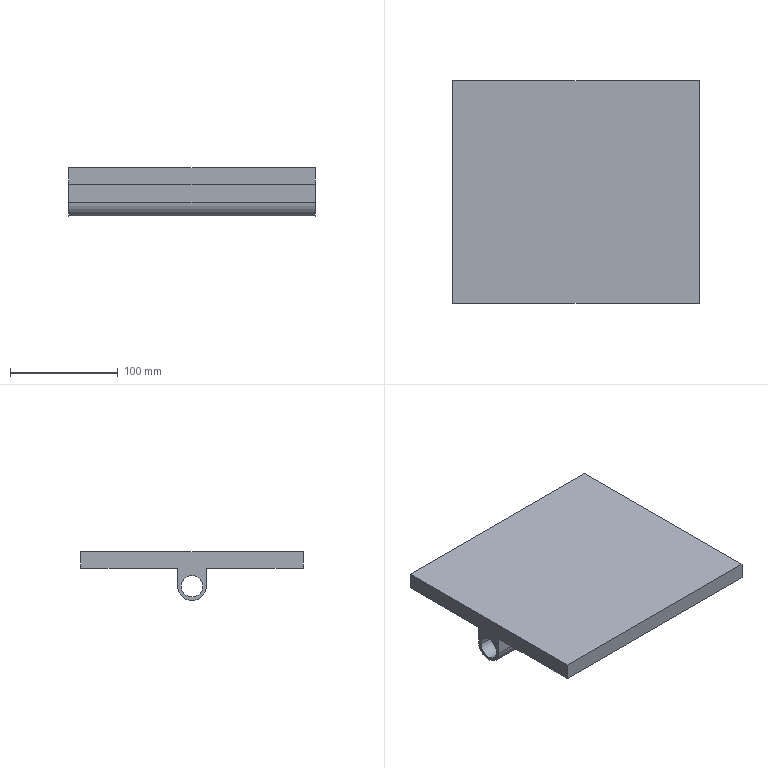Part | STEP file | 1 solid | 12 faces | box 229 x 206.363 x 45.369 mm | volume 819761 mm3 | plane 9 | cylinder 3 | commonest cylinder face diameters 20 x2 26.524 x1
STEP:
#1=CARTESIAN_POINT('',(0.,0.,0.));
#2=DIRECTION('',(0.,0.,1.));
#3=DIRECTION('',(1.,0.,0.));
#4=AXIS2_PLACEMENT_3D('',#1,#2,#3);
#5=CARTESIAN_POINT('',(226.149,563.5,104.906));
#6=VERTEX_POINT('',#5);
#7=CARTESIAN_POINT('',(455.149,563.5,104.906));
#8=VERTEX_POINT('',#7);
#9=CARTESIAN_POINT('',(226.149,563.5,104.906));
#10=DIRECTION('',(1.,0.,0.));
#11=VECTOR('',#10,1.);
#12=LINE('',#9,#11);
#13=CARTESIAN_POINT('',(226.149,553.5,104.906));
#14=DIRECTION('',(1.,0.,0.));
#15=DIRECTION('',(0.,1.,0.));
#16=AXIS2_PLACEMENT_3D('',#13,#14,#15);
#17=CYLINDRICAL_SURFACE('',#16,10.);
#18=CARTESIAN_POINT('',(6.283,0.));
#19=DIRECTION('',(0.,1.));
#20=VECTOR('',#19,1.);
#21=LINE('',#18,#20);
#22=(GEOMETRIC_REPRESENTATION_CONTEXT(2)PARAMETRIC_REPRESENTATION_CONTEXT()REPRESENTATION_CONTEXT('',''));
#23=DEFINITIONAL_REPRESENTATION('',(#21),#22);
#24=PCURVE('',#17,#23);
#25=CARTESIAN_POINT('',(226.149,553.5,104.906));
#26=DIRECTION('',(1.,0.,0.));
#27=DIRECTION('',(0.,1.,0.));
#28=AXIS2_PLACEMENT_3D('',#25,#26,#27);
#29=CYLINDRICAL_SURFACE('',#28,10.);
#30=CARTESIAN_POINT('',(0.,0.));
#31=DIRECTION('',(0.,1.));
#32=VECTOR('',#31,1.);
#33=LINE('',#30,#32);
#34=(GEOMETRIC_REPRESENTATION_CONTEXT(2)PARAMETRIC_REPRESENTATION_CONTEXT()REPRESENTATION_CONTEXT('',''));
#35=DEFINITIONAL_REPRESENTATION('',(#33),#34);
#36=PCURVE('',#29,#35);
#37=SURFACE_CURVE('',#12,(#24,#36),.PCURVE_S1.);
#38=EDGE_CURVE('',#6,#8,#37,.T.);
#39=ORIENTED_EDGE('',*,*,#38,.T.);
#40=CARTESIAN_POINT('',(455.149,543.5,104.906));
#41=VERTEX_POINT('',#40);
#42=CARTESIAN_POINT('',(455.149,553.5,104.906));
#43=DIRECTION('',(-1.,0.,0.));
#44=DIRECTION('',(0.,-1.,0.));
#45=AXIS2_PLACEMENT_3D('',#42,#43,#44);
#46=CIRCLE('',#45,10.);
#47=CARTESIAN_POINT('',(9.425,229.));
#48=DIRECTION('',(-1.,0.));
#49=VECTOR('',#48,1.);
#50=LINE('',#47,#49);
#51=(GEOMETRIC_REPRESENTATION_CONTEXT(2)PARAMETRIC_REPRESENTATION_CONTEXT()REPRESENTATION_CONTEXT('',''));
#52=DEFINITIONAL_REPRESENTATION('',(#50),#51);
#53=PCURVE('',#17,#52);
#54=CARTESIAN_POINT('',(455.149,553.5,104.906));
#55=DIRECTION('',(-1.,0.,0.));
#56=DIRECTION('',(0.,-1.,0.));
#57=AXIS2_PLACEMENT_3D('',#54,#55,#56);
#58=PLANE('',#57);
#59=CARTESIAN_POINT('',(0.,0.));
#60=DIRECTION('',(1.,0.));
#61=AXIS2_PLACEMENT_2D('',#59,#60);
#62=CIRCLE('',#61,10.);
#63=(GEOMETRIC_REPRESENTATION_CONTEXT(2)PARAMETRIC_REPRESENTATION_CONTEXT()REPRESENTATION_CONTEXT('',''));
#64=DEFINITIONAL_REPRESENTATION('',(#62),#63);
#65=PCURVE('',#58,#64);
#66=SURFACE_CURVE('',#46,(#53,#65),.PCURVE_S1.);
#67=EDGE_CURVE('',#8,#41,#66,.T.);
#68=ORIENTED_EDGE('',*,*,#67,.T.);
#69=CARTESIAN_POINT('',(226.149,543.5,104.906));
#70=VERTEX_POINT('',#69);
#71=CARTESIAN_POINT('',(226.149,543.5,104.906));
#72=DIRECTION('',(1.,0.,0.));
#73=VECTOR('',#72,1.);
#74=LINE('',#71,#73);
#75=CARTESIAN_POINT('',(3.142,0.));
#76=DIRECTION('',(0.,1.));
#77=VECTOR('',#76,1.);
#78=LINE('',#75,#77);
#79=(GEOMETRIC_REPRESENTATION_CONTEXT(2)PARAMETRIC_REPRESENTATION_CONTEXT()REPRESENTATION_CONTEXT('',''));
#80=DEFINITIONAL_REPRESENTATION('',(#78),#79);
#81=PCURVE('',#17,#80);
#82=CARTESIAN_POINT('',(3.142,0.));
#83=DIRECTION('',(0.,1.));
#84=VECTOR('',#83,1.);
#85=LINE('',#82,#84);
#86=(GEOMETRIC_REPRESENTATION_CONTEXT(2)PARAMETRIC_REPRESENTATION_CONTEXT()REPRESENTATION_CONTEXT('',''));
#87=DEFINITIONAL_REPRESENTATION('',(#85),#86);
#88=PCURVE('',#29,#87);
#89=SURFACE_CURVE('',#74,(#81,#88),.PCURVE_S1.);
#90=EDGE_CURVE('',#70,#41,#89,.T.);
#91=ORIENTED_EDGE('',*,*,#90,.F.);
#92=CARTESIAN_POINT('',(226.149,553.5,104.906));
#93=DIRECTION('',(-1.,0.,0.));
#94=DIRECTION('',(0.,-1.,0.));
#95=AXIS2_PLACEMENT_3D('',#92,#93,#94);
#96=CIRCLE('',#95,10.);
#97=CARTESIAN_POINT('',(9.425,0.));
#98=DIRECTION('',(-1.,0.));
#99=VECTOR('',#98,1.);
#100=LINE('',#97,#99);
#101=(GEOMETRIC_REPRESENTATION_CONTEXT(2)PARAMETRIC_REPRESENTATION_CONTEXT()REPRESENTATION_CONTEXT('',''));
#102=DEFINITIONAL_REPRESENTATION('',(#100),#101);
#103=PCURVE('',#17,#102);
#104=CARTESIAN_POINT('',(226.149,553.5,104.906));
#105=DIRECTION('',(-1.,0.,0.));
#106=DIRECTION('',(0.,-1.,0.));
#107=AXIS2_PLACEMENT_3D('',#104,#105,#106);
#108=PLANE('',#107);
#109=CARTESIAN_POINT('',(0.,0.));
#110=DIRECTION('',(1.,0.));
#111=AXIS2_PLACEMENT_2D('',#109,#110);
#112=CIRCLE('',#111,10.);
#113=(GEOMETRIC_REPRESENTATION_CONTEXT(2)PARAMETRIC_REPRESENTATION_CONTEXT()REPRESENTATION_CONTEXT('',''));
#114=DEFINITIONAL_REPRESENTATION('',(#112),#113);
#115=PCURVE('',#108,#114);
#116=SURFACE_CURVE('',#96,(#103,#115),.PCURVE_S1.);
#117=EDGE_CURVE('',#6,#70,#116,.T.);
#118=ORIENTED_EDGE('',*,*,#117,.F.);
#119=EDGE_LOOP('',(#39,#68,#91,#118));
#120=FACE_BOUND('',#119,.F.);
#121=ADVANCED_FACE('',(#120),#17,.F.);
#122=CARTESIAN_POINT('',(226.149,656.681,121.632));
#123=VERTEX_POINT('',#122);
#124=CARTESIAN_POINT('',(226.149,566.762,121.632));
#125=VERTEX_POINT('',#124);
#126=CARTESIAN_POINT('',(226.149,656.681,121.632));
#127=DIRECTION('',(0.,-1.,0.));
#128=VECTOR('',#127,1.);
#129=LINE('',#126,#128);
#130=CARTESIAN_POINT('',(-103.181,16.727));
#131=DIRECTION('',(1.,0.));
#132=VECTOR('',#131,1.);
#133=LINE('',#130,#132);
#134=(GEOMETRIC_REPRESENTATION_CONTEXT(2)PARAMETRIC_REPRESENTATION_CONTEXT()REPRESENTATION_CONTEXT('',''));
#135=DEFINITIONAL_REPRESENTATION('',(#133),#134);
#136=PCURVE('',#108,#135);
#137=CARTESIAN_POINT('',(226.149,656.681,121.632));
#138=DIRECTION('',(0.,0.,1.));
#139=DIRECTION('',(0.,-1.,0.));
#140=AXIS2_PLACEMENT_3D('',#137,#138,#139);
#141=PLANE('',#140);
#142=CARTESIAN_POINT('',(0.,0.));
#143=DIRECTION('',(1.,0.));
#144=VECTOR('',#143,1.);
#145=LINE('',#142,#144);
#146=(GEOMETRIC_REPRESENTATION_CONTEXT(2)PARAMETRIC_REPRESENTATION_CONTEXT()REPRESENTATION_CONTEXT('',''));
#147=DEFINITIONAL_REPRESENTATION('',(#145),#146);
#148=PCURVE('',#141,#147);
#149=SURFACE_CURVE('',#129,(#136,#148),.PCURVE_S1.);
#150=EDGE_CURVE('',#123,#125,#149,.T.);
#151=ORIENTED_EDGE('',*,*,#150,.T.);
#152=CARTESIAN_POINT('',(226.149,566.762,104.906));
#153=VERTEX_POINT('',#152);
#154=CARTESIAN_POINT('',(226.149,566.762,104.906));
#155=DIRECTION('',(0.,0.,-1.));
#156=VECTOR('',#155,1.);
#157=LINE('',#154,#156);
#158=CARTESIAN_POINT('',(-13.262,0.));
#159=DIRECTION('',(0.,-1.));
#160=VECTOR('',#159,1.);
#161=LINE('',#158,#160);
#162=(GEOMETRIC_REPRESENTATION_CONTEXT(2)PARAMETRIC_REPRESENTATION_CONTEXT()REPRESENTATION_CONTEXT('',''));
#163=DEFINITIONAL_REPRESENTATION('',(#161),#162);
#164=PCURVE('',#108,#163);
#165=CARTESIAN_POINT('',(226.149,566.762,104.906));
#166=DIRECTION('',(0.,-1.,0.));
#167=DIRECTION('',(1.,0.,0.));
#168=AXIS2_PLACEMENT_3D('',#165,#166,#167);
#169=PLANE('',#168);
#170=CARTESIAN_POINT('',(0.,0.));
#171=DIRECTION('',(0.,-1.));
#172=VECTOR('',#171,1.);
#173=LINE('',#170,#172);
#174=(GEOMETRIC_REPRESENTATION_CONTEXT(2)PARAMETRIC_REPRESENTATION_CONTEXT()REPRESENTATION_CONTEXT('',''));
#175=DEFINITIONAL_REPRESENTATION('',(#173),#174);
#176=PCURVE('',#169,#175);
#177=SURFACE_CURVE('',#157,(#164,#176),.PCURVE_S1.);
#178=EDGE_CURVE('',#125,#153,#177,.T.);
#179=ORIENTED_EDGE('',*,*,#178,.T.);
#180=CARTESIAN_POINT('',(226.149,540.238,104.906));
#181=VERTEX_POINT('',#180);
#182=CARTESIAN_POINT('',(226.149,553.5,104.906));
#183=DIRECTION('',(-1.,0.,0.));
#184=DIRECTION('',(0.,-1.,0.));
#185=AXIS2_PLACEMENT_3D('',#182,#183,#184);
#186=CIRCLE('',#185,13.262);
#187=CARTESIAN_POINT('',(0.,0.));
#188=DIRECTION('',(1.,0.));
#189=AXIS2_PLACEMENT_2D('',#187,#188);
#190=CIRCLE('',#189,13.262);
#191=(GEOMETRIC_REPRESENTATION_CONTEXT(2)PARAMETRIC_REPRESENTATION_CONTEXT()REPRESENTATION_CONTEXT('',''));
#192=DEFINITIONAL_REPRESENTATION('',(#190),#191);
#193=PCURVE('',#108,#192);
#194=CARTESIAN_POINT('',(226.149,553.5,104.906));
#195=DIRECTION('',(1.,0.,0.));
#196=DIRECTION('',(0.,1.,0.));
#197=AXIS2_PLACEMENT_3D('',#194,#195,#196);
#198=CYLINDRICAL_SURFACE('',#197,13.262);
#199=CARTESIAN_POINT('',(9.425,0.));
#200=DIRECTION('',(-1.,0.));
#201=VECTOR('',#200,1.);
#202=LINE('',#199,#201);
#203=(GEOMETRIC_REPRESENTATION_CONTEXT(2)PARAMETRIC_REPRESENTATION_CONTEXT()REPRESENTATION_CONTEXT('',''));
#204=DEFINITIONAL_REPRESENTATION('',(#202),#203);
#205=PCURVE('',#198,#204);
#206=SURFACE_CURVE('',#186,(#193,#205),.PCURVE_S1.);
#207=EDGE_CURVE('',#153,#181,#206,.T.);
#208=ORIENTED_EDGE('',*,*,#207,.T.);
#209=CARTESIAN_POINT('',(226.149,540.238,121.632));
#210=VERTEX_POINT('',#209);
#211=CARTESIAN_POINT('',(226.149,540.238,104.906));
#212=DIRECTION('',(0.,0.,1.));
#213=VECTOR('',#212,1.);
#214=LINE('',#211,#213);
#215=CARTESIAN_POINT('',(13.262,0.));
#216=DIRECTION('',(0.,1.));
#217=VECTOR('',#216,1.);
#218=LINE('',#215,#217);
#219=(GEOMETRIC_REPRESENTATION_CONTEXT(2)PARAMETRIC_REPRESENTATION_CONTEXT()REPRESENTATION_CONTEXT('',''));
#220=DEFINITIONAL_REPRESENTATION('',(#218),#219);
#221=PCURVE('',#108,#220);
#222=CARTESIAN_POINT('',(226.149,540.238,104.906));
#223=DIRECTION('',(0.,1.,0.));
#224=DIRECTION('',(-1.,0.,0.));
#225=AXIS2_PLACEMENT_3D('',#222,#223,#224);
#226=PLANE('',#225);
#227=CARTESIAN_POINT('',(0.,0.));
#228=DIRECTION('',(0.,1.));
#229=VECTOR('',#228,1.);
#230=LINE('',#227,#229);
#231=(GEOMETRIC_REPRESENTATION_CONTEXT(2)PARAMETRIC_REPRESENTATION_CONTEXT()REPRESENTATION_CONTEXT('',''));
#232=DEFINITIONAL_REPRESENTATION('',(#230),#231);
#233=PCURVE('',#226,#232);
#234=SURFACE_CURVE('',#214,(#221,#233),.PCURVE_S1.);
#235=EDGE_CURVE('',#181,#210,#234,.T.);
#236=ORIENTED_EDGE('',*,*,#235,.T.);
#237=CARTESIAN_POINT('',(226.149,450.319,121.632));
#238=VERTEX_POINT('',#237);
#239=CARTESIAN_POINT('',(226.149,540.238,121.632));
#240=DIRECTION('',(0.,-1.,0.));
#241=VECTOR('',#240,1.);
#242=LINE('',#239,#241);
#243=CARTESIAN_POINT('',(13.262,16.727));
#244=DIRECTION('',(1.,0.));
#245=VECTOR('',#244,1.);
#246=LINE('',#243,#245);
#247=(GEOMETRIC_REPRESENTATION_CONTEXT(2)PARAMETRIC_REPRESENTATION_CONTEXT()REPRESENTATION_CONTEXT('',''));
#248=DEFINITIONAL_REPRESENTATION('',(#246),#247);
#249=PCURVE('',#108,#248);
#250=CARTESIAN_POINT('',(226.149,540.238,121.632));
#251=DIRECTION('',(0.,0.,1.));
#252=DIRECTION('',(0.,-1.,0.));
#253=AXIS2_PLACEMENT_3D('',#250,#251,#252);
#254=PLANE('',#253);
#255=CARTESIAN_POINT('',(0.,0.));
#256=DIRECTION('',(1.,0.));
#257=VECTOR('',#256,1.);
#258=LINE('',#255,#257);
#259=(GEOMETRIC_REPRESENTATION_CONTEXT(2)PARAMETRIC_REPRESENTATION_CONTEXT()REPRESENTATION_CONTEXT('',''));
#260=DEFINITIONAL_REPRESENTATION('',(#258),#259);
#261=PCURVE('',#254,#260);
#262=SURFACE_CURVE('',#242,(#249,#261),.PCURVE_S1.);
#263=EDGE_CURVE('',#210,#238,#262,.T.);
#264=ORIENTED_EDGE('',*,*,#263,.T.);
#265=CARTESIAN_POINT('',(226.149,450.319,137.013));
#266=VERTEX_POINT('',#265);
#267=CARTESIAN_POINT('',(226.149,450.319,121.632));
#268=DIRECTION('',(0.,0.,1.));
#269=VECTOR('',#268,1.);
#270=LINE('',#267,#269);
#271=CARTESIAN_POINT('',(103.181,16.727));
#272=DIRECTION('',(0.,1.));
#273=VECTOR('',#272,1.);
#274=LINE('',#271,#273);
#275=(GEOMETRIC_REPRESENTATION_CONTEXT(2)PARAMETRIC_REPRESENTATION_CONTEXT()REPRESENTATION_CONTEXT('',''));
#276=DEFINITIONAL_REPRESENTATION('',(#274),#275);
#277=PCURVE('',#108,#276);
#278=CARTESIAN_POINT('',(226.149,450.319,121.632));
#279=DIRECTION('',(0.,1.,0.));
#280=DIRECTION('',(-1.,0.,0.));
#281=AXIS2_PLACEMENT_3D('',#278,#279,#280);
#282=PLANE('',#281);
#283=CARTESIAN_POINT('',(0.,0.));
#284=DIRECTION('',(0.,1.));
#285=VECTOR('',#284,1.);
#286=LINE('',#283,#285);
#287=(GEOMETRIC_REPRESENTATION_CONTEXT(2)PARAMETRIC_REPRESENTATION_CONTEXT()REPRESENTATION_CONTEXT('',''));
#288=DEFINITIONAL_REPRESENTATION('',(#286),#287);
#289=PCURVE('',#282,#288);
#290=SURFACE_CURVE('',#270,(#277,#289),.PCURVE_S1.);
#291=EDGE_CURVE('',#238,#266,#290,.T.);
#292=ORIENTED_EDGE('',*,*,#291,.T.);
#293=CARTESIAN_POINT('',(226.149,656.681,137.013));
#294=VERTEX_POINT('',#293);
#295=CARTESIAN_POINT('',(226.149,656.681,137.013));
#296=DIRECTION('',(0.,1.,0.));
#297=VECTOR('',#296,1.);
#298=LINE('',#295,#297);
#299=CARTESIAN_POINT('',(-103.181,32.107));
#300=DIRECTION('',(-1.,0.));
#301=VECTOR('',#300,1.);
#302=LINE('',#299,#301);
#303=(GEOMETRIC_REPRESENTATION_CONTEXT(2)PARAMETRIC_REPRESENTATION_CONTEXT()REPRESENTATION_CONTEXT('',''));
#304=DEFINITIONAL_REPRESENTATION('',(#302),#303);
#305=PCURVE('',#108,#304);
#306=CARTESIAN_POINT('',(226.149,656.681,137.013));
#307=DIRECTION('',(0.,0.,-1.));
#308=DIRECTION('',(-1.,0.,0.));
#309=AXIS2_PLACEMENT_3D('',#306,#307,#308);
#310=PLANE('',#309);
#311=CARTESIAN_POINT('',(0.,0.));
#312=DIRECTION('',(0.,1.));
#313=VECTOR('',#312,1.);
#314=LINE('',#311,#313);
#315=(GEOMETRIC_REPRESENTATION_CONTEXT(2)PARAMETRIC_REPRESENTATION_CONTEXT()REPRESENTATION_CONTEXT('',''));
#316=DEFINITIONAL_REPRESENTATION('',(#314),#315);
#317=PCURVE('',#310,#316);
#318=SURFACE_CURVE('',#298,(#305,#317),.PCURVE_S1.);
#319=EDGE_CURVE('',#266,#294,#318,.T.);
#320=ORIENTED_EDGE('',*,*,#319,.T.);
#321=CARTESIAN_POINT('',(226.149,656.681,121.632));
#322=DIRECTION('',(0.,0.,-1.));
#323=VECTOR('',#322,1.);
#324=LINE('',#321,#323);
#325=CARTESIAN_POINT('',(-103.181,16.727));
#326=DIRECTION('',(0.,-1.));
#327=VECTOR('',#326,1.);
#328=LINE('',#325,#327);
#329=(GEOMETRIC_REPRESENTATION_CONTEXT(2)PARAMETRIC_REPRESENTATION_CONTEXT()REPRESENTATION_CONTEXT('',''));
#330=DEFINITIONAL_REPRESENTATION('',(#328),#329);
#331=PCURVE('',#108,#330);
#332=CARTESIAN_POINT('',(226.149,656.681,121.632));
#333=DIRECTION('',(0.,-1.,0.));
#334=DIRECTION('',(1.,0.,0.));
#335=AXIS2_PLACEMENT_3D('',#332,#333,#334);
#336=PLANE('',#335);
#337=CARTESIAN_POINT('',(0.,0.));
#338=DIRECTION('',(0.,-1.));
#339=VECTOR('',#338,1.);
#340=LINE('',#337,#339);
#341=(GEOMETRIC_REPRESENTATION_CONTEXT(2)PARAMETRIC_REPRESENTATION_CONTEXT()REPRESENTATION_CONTEXT('',''));
#342=DEFINITIONAL_REPRESENTATION('',(#340),#341);
#343=PCURVE('',#336,#342);
#344=SURFACE_CURVE('',#324,(#331,#343),.PCURVE_S1.);
#345=EDGE_CURVE('',#294,#123,#344,.T.);
#346=ORIENTED_EDGE('',*,*,#345,.T.);
#347=EDGE_LOOP('',(#151,#179,#208,#236,#264,#292,#320,#346));
#348=FACE_BOUND('',#347,.T.);
#349=ORIENTED_EDGE('',*,*,#117,.F.);
#350=CARTESIAN_POINT('',(226.149,553.5,104.906));
#351=DIRECTION('',(-1.,0.,0.));
#352=DIRECTION('',(0.,-1.,0.));
#353=AXIS2_PLACEMENT_3D('',#350,#351,#352);
#354=CIRCLE('',#353,10.);
#355=CARTESIAN_POINT('',(0.,0.));
#356=DIRECTION('',(1.,0.));
#357=AXIS2_PLACEMENT_2D('',#355,#356);
#358=CIRCLE('',#357,10.);
#359=(GEOMETRIC_REPRESENTATION_CONTEXT(2)PARAMETRIC_REPRESENTATION_CONTEXT()REPRESENTATION_CONTEXT('',''));
#360=DEFINITIONAL_REPRESENTATION('',(#358),#359);
#361=PCURVE('',#108,#360);
#362=CARTESIAN_POINT('',(3.142,0.));
#363=DIRECTION('',(-1.,0.));
#364=VECTOR('',#363,1.);
#365=LINE('',#362,#364);
#366=(GEOMETRIC_REPRESENTATION_CONTEXT(2)PARAMETRIC_REPRESENTATION_CONTEXT()REPRESENTATION_CONTEXT('',''));
#367=DEFINITIONAL_REPRESENTATION('',(#365),#366);
#368=PCURVE('',#29,#367);
#369=SURFACE_CURVE('',#354,(#361,#368),.PCURVE_S1.);
#370=EDGE_CURVE('',#70,#6,#369,.T.);
#371=ORIENTED_EDGE('',*,*,#370,.F.);
#372=EDGE_LOOP('',(#349,#371));
#373=FACE_BOUND('',#372,.T.);
#374=ADVANCED_FACE('',(#348,#373),#108,.T.);
#375=CARTESIAN_POINT('',(455.149,656.681,121.632));
#376=VERTEX_POINT('',#375);
#377=CARTESIAN_POINT('',(455.149,566.762,121.632));
#378=VERTEX_POINT('',#377);
#379=CARTESIAN_POINT('',(455.149,656.681,121.632));
#380=DIRECTION('',(0.,-1.,0.));
#381=VECTOR('',#380,1.);
#382=LINE('',#379,#381);
#383=CARTESIAN_POINT('',(-103.181,16.727));
#384=DIRECTION('',(1.,0.));
#385=VECTOR('',#384,1.);
#386=LINE('',#383,#385);
#387=(GEOMETRIC_REPRESENTATION_CONTEXT(2)PARAMETRIC_REPRESENTATION_CONTEXT()REPRESENTATION_CONTEXT('',''));
#388=DEFINITIONAL_REPRESENTATION('',(#386),#387);
#389=PCURVE('',#58,#388);
#390=CARTESIAN_POINT('',(0.,229.));
#391=DIRECTION('',(1.,0.));
#392=VECTOR('',#391,1.);
#393=LINE('',#390,#392);
#394=(GEOMETRIC_REPRESENTATION_CONTEXT(2)PARAMETRIC_REPRESENTATION_CONTEXT()REPRESENTATION_CONTEXT('',''));
#395=DEFINITIONAL_REPRESENTATION('',(#393),#394);
#396=PCURVE('',#141,#395);
#397=SURFACE_CURVE('',#382,(#389,#396),.PCURVE_S1.);
#398=EDGE_CURVE('',#376,#378,#397,.T.);
#399=ORIENTED_EDGE('',*,*,#398,.F.);
#400=CARTESIAN_POINT('',(455.149,656.681,137.013));
#401=VERTEX_POINT('',#400);
#402=CARTESIAN_POINT('',(455.149,656.681,121.632));
#403=DIRECTION('',(0.,0.,-1.));
#404=VECTOR('',#403,1.);
#405=LINE('',#402,#404);
#406=CARTESIAN_POINT('',(-103.181,16.727));
#407=DIRECTION('',(0.,-1.));
#408=VECTOR('',#407,1.);
#409=LINE('',#406,#408);
#410=(GEOMETRIC_REPRESENTATION_CONTEXT(2)PARAMETRIC_REPRESENTATION_CONTEXT()REPRESENTATION_CONTEXT('',''));
#411=DEFINITIONAL_REPRESENTATION('',(#409),#410);
#412=PCURVE('',#58,#411);
#413=CARTESIAN_POINT('',(229.,0.));
#414=DIRECTION('',(0.,-1.));
#415=VECTOR('',#414,1.);
#416=LINE('',#413,#415);
#417=(GEOMETRIC_REPRESENTATION_CONTEXT(2)PARAMETRIC_REPRESENTATION_CONTEXT()REPRESENTATION_CONTEXT('',''));
#418=DEFINITIONAL_REPRESENTATION('',(#416),#417);
#419=PCURVE('',#336,#418);
#420=SURFACE_CURVE('',#405,(#412,#419),.PCURVE_S1.);
#421=EDGE_CURVE('',#401,#376,#420,.T.);
#422=ORIENTED_EDGE('',*,*,#421,.F.);
#423=CARTESIAN_POINT('',(455.149,450.319,137.013));
#424=VERTEX_POINT('',#423);
#425=CARTESIAN_POINT('',(455.149,656.681,137.013));
#426=DIRECTION('',(0.,1.,0.));
#427=VECTOR('',#426,1.);
#428=LINE('',#425,#427);
#429=CARTESIAN_POINT('',(-103.181,32.107));
#430=DIRECTION('',(-1.,0.));
#431=VECTOR('',#430,1.);
#432=LINE('',#429,#431);
#433=(GEOMETRIC_REPRESENTATION_CONTEXT(2)PARAMETRIC_REPRESENTATION_CONTEXT()REPRESENTATION_CONTEXT('',''));
#434=DEFINITIONAL_REPRESENTATION('',(#432),#433);
#435=PCURVE('',#58,#434);
#436=CARTESIAN_POINT('',(-229.,0.));
#437=DIRECTION('',(0.,1.));
#438=VECTOR('',#437,1.);
#439=LINE('',#436,#438);
#440=(GEOMETRIC_REPRESENTATION_CONTEXT(2)PARAMETRIC_REPRESENTATION_CONTEXT()REPRESENTATION_CONTEXT('',''));
#441=DEFINITIONAL_REPRESENTATION('',(#439),#440);
#442=PCURVE('',#310,#441);
#443=SURFACE_CURVE('',#428,(#435,#442),.PCURVE_S1.);
#444=EDGE_CURVE('',#424,#401,#443,.T.);
#445=ORIENTED_EDGE('',*,*,#444,.F.);
#446=CARTESIAN_POINT('',(455.149,450.319,121.632));
#447=VERTEX_POINT('',#446);
#448=CARTESIAN_POINT('',(455.149,450.319,121.632));
#449=DIRECTION('',(0.,0.,1.));
#450=VECTOR('',#449,1.);
#451=LINE('',#448,#450);
#452=CARTESIAN_POINT('',(103.181,16.727));
#453=DIRECTION('',(0.,1.));
#454=VECTOR('',#453,1.);
#455=LINE('',#452,#454);
#456=(GEOMETRIC_REPRESENTATION_CONTEXT(2)PARAMETRIC_REPRESENTATION_CONTEXT()REPRESENTATION_CONTEXT('',''));
#457=DEFINITIONAL_REPRESENTATION('',(#455),#456);
#458=PCURVE('',#58,#457);
#459=CARTESIAN_POINT('',(-229.,0.));
#460=DIRECTION('',(0.,1.));
#461=VECTOR('',#460,1.);
#462=LINE('',#459,#461);
#463=(GEOMETRIC_REPRESENTATION_CONTEXT(2)PARAMETRIC_REPRESENTATION_CONTEXT()REPRESENTATION_CONTEXT('',''));
#464=DEFINITIONAL_REPRESENTATION('',(#462),#463);
#465=PCURVE('',#282,#464);
#466=SURFACE_CURVE('',#451,(#458,#465),.PCURVE_S1.);
#467=EDGE_CURVE('',#447,#424,#466,.T.);
#468=ORIENTED_EDGE('',*,*,#467,.F.);
#469=CARTESIAN_POINT('',(455.149,540.238,121.632));
#470=VERTEX_POINT('',#469);
#471=CARTESIAN_POINT('',(455.149,540.238,121.632));
#472=DIRECTION('',(0.,-1.,0.));
#473=VECTOR('',#472,1.);
#474=LINE('',#471,#473);
#475=CARTESIAN_POINT('',(13.262,16.727));
#476=DIRECTION('',(1.,0.));
#477=VECTOR('',#476,1.);
#478=LINE('',#475,#477);
#479=(GEOMETRIC_REPRESENTATION_CONTEXT(2)PARAMETRIC_REPRESENTATION_CONTEXT()REPRESENTATION_CONTEXT('',''));
#480=DEFINITIONAL_REPRESENTATION('',(#478),#479);
#481=PCURVE('',#58,#480);
#482=CARTESIAN_POINT('',(0.,229.));
#483=DIRECTION('',(1.,0.));
#484=VECTOR('',#483,1.);
#485=LINE('',#482,#484);
#486=(GEOMETRIC_REPRESENTATION_CONTEXT(2)PARAMETRIC_REPRESENTATION_CONTEXT()REPRESENTATION_CONTEXT('',''));
#487=DEFINITIONAL_REPRESENTATION('',(#485),#486);
#488=PCURVE('',#254,#487);
#489=SURFACE_CURVE('',#474,(#481,#488),.PCURVE_S1.);
#490=EDGE_CURVE('',#470,#447,#489,.T.);
#491=ORIENTED_EDGE('',*,*,#490,.F.);
#492=CARTESIAN_POINT('',(455.149,540.238,104.906));
#493=VERTEX_POINT('',#492);
#494=CARTESIAN_POINT('',(455.149,540.238,104.906));
#495=DIRECTION('',(0.,0.,1.));
#496=VECTOR('',#495,1.);
#497=LINE('',#494,#496);
#498=CARTESIAN_POINT('',(13.262,0.));
#499=DIRECTION('',(0.,1.));
#500=VECTOR('',#499,1.);
#501=LINE('',#498,#500);
#502=(GEOMETRIC_REPRESENTATION_CONTEXT(2)PARAMETRIC_REPRESENTATION_CONTEXT()REPRESENTATION_CONTEXT('',''));
#503=DEFINITIONAL_REPRESENTATION('',(#501),#502);
#504=PCURVE('',#58,#503);
#505=CARTESIAN_POINT('',(-229.,0.));
#506=DIRECTION('',(0.,1.));
#507=VECTOR('',#506,1.);
#508=LINE('',#505,#507);
#509=(GEOMETRIC_REPRESENTATION_CONTEXT(2)PARAMETRIC_REPRESENTATION_CONTEXT()REPRESENTATION_CONTEXT('',''));
#510=DEFINITIONAL_REPRESENTATION('',(#508),#509);
#511=PCURVE('',#226,#510);
#512=SURFACE_CURVE('',#497,(#504,#511),.PCURVE_S1.);
#513=EDGE_CURVE('',#493,#470,#512,.T.);
#514=ORIENTED_EDGE('',*,*,#513,.F.);
#515=CARTESIAN_POINT('',(455.149,566.762,104.906));
#516=VERTEX_POINT('',#515);
#517=CARTESIAN_POINT('',(455.149,553.5,104.906));
#518=DIRECTION('',(-1.,0.,0.));
#519=DIRECTION('',(0.,-1.,0.));
#520=AXIS2_PLACEMENT_3D('',#517,#518,#519);
#521=CIRCLE('',#520,13.262);
#522=CARTESIAN_POINT('',(0.,0.));
#523=DIRECTION('',(1.,0.));
#524=AXIS2_PLACEMENT_2D('',#522,#523);
#525=CIRCLE('',#524,13.262);
#526=(GEOMETRIC_REPRESENTATION_CONTEXT(2)PARAMETRIC_REPRESENTATION_CONTEXT()REPRESENTATION_CONTEXT('',''));
#527=DEFINITIONAL_REPRESENTATION('',(#525),#526);
#528=PCURVE('',#58,#527);
#529=CARTESIAN_POINT('',(9.425,229.));
#530=DIRECTION('',(-1.,0.));
#531=VECTOR('',#530,1.);
#532=LINE('',#529,#531);
#533=(GEOMETRIC_REPRESENTATION_CONTEXT(2)PARAMETRIC_REPRESENTATION_CONTEXT()REPRESENTATION_CONTEXT('',''));
#534=DEFINITIONAL_REPRESENTATION('',(#532),#533);
#535=PCURVE('',#198,#534);
#536=SURFACE_CURVE('',#521,(#528,#535),.PCURVE_S1.);
#537=EDGE_CURVE('',#516,#493,#536,.T.);
#538=ORIENTED_EDGE('',*,*,#537,.F.);
#539=CARTESIAN_POINT('',(455.149,566.762,104.906));
#540=DIRECTION('',(0.,0.,-1.));
#541=VECTOR('',#540,1.);
#542=LINE('',#539,#541);
#543=CARTESIAN_POINT('',(-13.262,0.));
#544=DIRECTION('',(0.,-1.));
#545=VECTOR('',#544,1.);
#546=LINE('',#543,#545);
#547=(GEOMETRIC_REPRESENTATION_CONTEXT(2)PARAMETRIC_REPRESENTATION_CONTEXT()REPRESENTATION_CONTEXT('',''));
#548=DEFINITIONAL_REPRESENTATION('',(#546),#547);
#549=PCURVE('',#58,#548);
#550=CARTESIAN_POINT('',(229.,0.));
#551=DIRECTION('',(0.,-1.));
#552=VECTOR('',#551,1.);
#553=LINE('',#550,#552);
#554=(GEOMETRIC_REPRESENTATION_CONTEXT(2)PARAMETRIC_REPRESENTATION_CONTEXT()REPRESENTATION_CONTEXT('',''));
#555=DEFINITIONAL_REPRESENTATION('',(#553),#554);
#556=PCURVE('',#169,#555);
#557=SURFACE_CURVE('',#542,(#549,#556),.PCURVE_S1.);
#558=EDGE_CURVE('',#378,#516,#557,.T.);
#559=ORIENTED_EDGE('',*,*,#558,.F.);
#560=EDGE_LOOP('',(#399,#422,#445,#468,#491,#514,#538,#559));
#561=FACE_BOUND('',#560,.T.);
#562=ORIENTED_EDGE('',*,*,#67,.T.);
#563=CARTESIAN_POINT('',(455.149,553.5,104.906));
#564=DIRECTION('',(-1.,0.,0.));
#565=DIRECTION('',(0.,-1.,0.));
#566=AXIS2_PLACEMENT_3D('',#563,#564,#565);
#567=CIRCLE('',#566,10.);
#568=CARTESIAN_POINT('',(0.,0.));
#569=DIRECTION('',(1.,0.));
#570=AXIS2_PLACEMENT_2D('',#568,#569);
#571=CIRCLE('',#570,10.);
#572=(GEOMETRIC_REPRESENTATION_CONTEXT(2)PARAMETRIC_REPRESENTATION_CONTEXT()REPRESENTATION_CONTEXT('',''));
#573=DEFINITIONAL_REPRESENTATION('',(#571),#572);
#574=PCURVE('',#58,#573);
#575=CARTESIAN_POINT('',(3.142,229.));
#576=DIRECTION('',(-1.,0.));
#577=VECTOR('',#576,1.);
#578=LINE('',#575,#577);
#579=(GEOMETRIC_REPRESENTATION_CONTEXT(2)PARAMETRIC_REPRESENTATION_CONTEXT()REPRESENTATION_CONTEXT('',''));
#580=DEFINITIONAL_REPRESENTATION('',(#578),#579);
#581=PCURVE('',#29,#580);
#582=SURFACE_CURVE('',#567,(#574,#581),.PCURVE_S1.);
#583=EDGE_CURVE('',#41,#8,#582,.T.);
#584=ORIENTED_EDGE('',*,*,#583,.T.);
#585=EDGE_LOOP('',(#562,#584));
#586=FACE_BOUND('',#585,.T.);
#587=ADVANCED_FACE('',(#561,#586),#58,.F.);
#588=ORIENTED_EDGE('',*,*,#398,.T.);
#589=CARTESIAN_POINT('',(226.149,566.762,121.632));
#590=DIRECTION('',(1.,0.,0.));
#591=VECTOR('',#590,1.);
#592=LINE('',#589,#591);
#593=CARTESIAN_POINT('',(89.919,0.));
#594=DIRECTION('',(0.,1.));
#595=VECTOR('',#594,1.);
#596=LINE('',#593,#595);
#597=(GEOMETRIC_REPRESENTATION_CONTEXT(2)PARAMETRIC_REPRESENTATION_CONTEXT()REPRESENTATION_CONTEXT('',''));
#598=DEFINITIONAL_REPRESENTATION('',(#596),#597);
#599=PCURVE('',#141,#598);
#600=CARTESIAN_POINT('',(0.,16.727));
#601=DIRECTION('',(1.,0.));
#602=VECTOR('',#601,1.);
#603=LINE('',#600,#602);
#604=(GEOMETRIC_REPRESENTATION_CONTEXT(2)PARAMETRIC_REPRESENTATION_CONTEXT()REPRESENTATION_CONTEXT('',''));
#605=DEFINITIONAL_REPRESENTATION('',(#603),#604);
#606=PCURVE('',#169,#605);
#607=SURFACE_CURVE('',#592,(#599,#606),.PCURVE_S1.);
#608=EDGE_CURVE('',#125,#378,#607,.T.);
#609=ORIENTED_EDGE('',*,*,#608,.F.);
#610=ORIENTED_EDGE('',*,*,#150,.F.);
#611=CARTESIAN_POINT('',(226.149,656.681,121.632));
#612=DIRECTION('',(1.,0.,0.));
#613=VECTOR('',#612,1.);
#614=LINE('',#611,#613);
#615=CARTESIAN_POINT('',(0.,0.));
#616=DIRECTION('',(0.,1.));
#617=VECTOR('',#616,1.);
#618=LINE('',#615,#617);
#619=(GEOMETRIC_REPRESENTATION_CONTEXT(2)PARAMETRIC_REPRESENTATION_CONTEXT()REPRESENTATION_CONTEXT('',''));
#620=DEFINITIONAL_REPRESENTATION('',(#618),#619);
#621=PCURVE('',#141,#620);
#622=CARTESIAN_POINT('',(0.,0.));
#623=DIRECTION('',(1.,0.));
#624=VECTOR('',#623,1.);
#625=LINE('',#622,#624);
#626=(GEOMETRIC_REPRESENTATION_CONTEXT(2)PARAMETRIC_REPRESENTATION_CONTEXT()REPRESENTATION_CONTEXT('',''));
#627=DEFINITIONAL_REPRESENTATION('',(#625),#626);
#628=PCURVE('',#336,#627);
#629=SURFACE_CURVE('',#614,(#621,#628),.PCURVE_S1.);
#630=EDGE_CURVE('',#123,#376,#629,.T.);
#631=ORIENTED_EDGE('',*,*,#630,.T.);
#632=EDGE_LOOP('',(#588,#609,#610,#631));
#633=FACE_BOUND('',#632,.T.);
#634=ADVANCED_FACE('',(#633),#141,.F.);
#635=ORIENTED_EDGE('',*,*,#558,.T.);
#636=CARTESIAN_POINT('',(226.149,566.762,104.906));
#637=DIRECTION('',(1.,0.,0.));
#638=VECTOR('',#637,1.);
#639=LINE('',#636,#638);
#640=CARTESIAN_POINT('',(0.,0.));
#641=DIRECTION('',(1.,0.));
#642=VECTOR('',#641,1.);
#643=LINE('',#640,#642);
#644=(GEOMETRIC_REPRESENTATION_CONTEXT(2)PARAMETRIC_REPRESENTATION_CONTEXT()REPRESENTATION_CONTEXT('',''));
#645=DEFINITIONAL_REPRESENTATION('',(#643),#644);
#646=PCURVE('',#169,#645);
#647=CARTESIAN_POINT('',(6.283,0.));
#648=DIRECTION('',(0.,1.));
#649=VECTOR('',#648,1.);
#650=LINE('',#647,#649);
#651=(GEOMETRIC_REPRESENTATION_CONTEXT(2)PARAMETRIC_REPRESENTATION_CONTEXT()REPRESENTATION_CONTEXT('',''));
#652=DEFINITIONAL_REPRESENTATION('',(#650),#651);
#653=PCURVE('',#198,#652);
#654=SURFACE_CURVE('',#639,(#646,#653),.PCURVE_S1.);
#655=EDGE_CURVE('',#153,#516,#654,.T.);
#656=ORIENTED_EDGE('',*,*,#655,.F.);
#657=ORIENTED_EDGE('',*,*,#178,.F.);
#658=ORIENTED_EDGE('',*,*,#608,.T.);
#659=EDGE_LOOP('',(#635,#656,#657,#658));
#660=FACE_BOUND('',#659,.T.);
#661=ADVANCED_FACE('',(#660),#169,.F.);
#662=ORIENTED_EDGE('',*,*,#537,.T.);
#663=CARTESIAN_POINT('',(226.149,540.238,104.906));
#664=DIRECTION('',(1.,0.,0.));
#665=VECTOR('',#664,1.);
#666=LINE('',#663,#665);
#667=CARTESIAN_POINT('',(3.142,0.));
#668=DIRECTION('',(0.,1.));
#669=VECTOR('',#668,1.);
#670=LINE('',#667,#669);
#671=(GEOMETRIC_REPRESENTATION_CONTEXT(2)PARAMETRIC_REPRESENTATION_CONTEXT()REPRESENTATION_CONTEXT('',''));
#672=DEFINITIONAL_REPRESENTATION('',(#670),#671);
#673=PCURVE('',#198,#672);
#674=CARTESIAN_POINT('',(0.,0.));
#675=DIRECTION('',(-1.,0.));
#676=VECTOR('',#675,1.);
#677=LINE('',#674,#676);
#678=(GEOMETRIC_REPRESENTATION_CONTEXT(2)PARAMETRIC_REPRESENTATION_CONTEXT()REPRESENTATION_CONTEXT('',''));
#679=DEFINITIONAL_REPRESENTATION('',(#677),#678);
#680=PCURVE('',#226,#679);
#681=SURFACE_CURVE('',#666,(#673,#680),.PCURVE_S1.);
#682=EDGE_CURVE('',#181,#493,#681,.T.);
#683=ORIENTED_EDGE('',*,*,#682,.F.);
#684=ORIENTED_EDGE('',*,*,#207,.F.);
#685=ORIENTED_EDGE('',*,*,#655,.T.);
#686=EDGE_LOOP('',(#662,#683,#684,#685));
#687=FACE_BOUND('',#686,.T.);
#688=ADVANCED_FACE('',(#687),#198,.T.);
#689=ORIENTED_EDGE('',*,*,#513,.T.);
#690=CARTESIAN_POINT('',(226.149,540.238,121.632));
#691=DIRECTION('',(1.,0.,0.));
#692=VECTOR('',#691,1.);
#693=LINE('',#690,#692);
#694=CARTESIAN_POINT('',(0.,16.727));
#695=DIRECTION('',(-1.,0.));
#696=VECTOR('',#695,1.);
#697=LINE('',#694,#696);
#698=(GEOMETRIC_REPRESENTATION_CONTEXT(2)PARAMETRIC_REPRESENTATION_CONTEXT()REPRESENTATION_CONTEXT('',''));
#699=DEFINITIONAL_REPRESENTATION('',(#697),#698);
#700=PCURVE('',#226,#699);
#701=CARTESIAN_POINT('',(0.,0.));
#702=DIRECTION('',(0.,1.));
#703=VECTOR('',#702,1.);
#704=LINE('',#701,#703);
#705=(GEOMETRIC_REPRESENTATION_CONTEXT(2)PARAMETRIC_REPRESENTATION_CONTEXT()REPRESENTATION_CONTEXT('',''));
#706=DEFINITIONAL_REPRESENTATION('',(#704),#705);
#707=PCURVE('',#254,#706);
#708=SURFACE_CURVE('',#693,(#700,#707),.PCURVE_S1.);
#709=EDGE_CURVE('',#210,#470,#708,.T.);
#710=ORIENTED_EDGE('',*,*,#709,.F.);
#711=ORIENTED_EDGE('',*,*,#235,.F.);
#712=ORIENTED_EDGE('',*,*,#682,.T.);
#713=EDGE_LOOP('',(#689,#710,#711,#712));
#714=FACE_BOUND('',#713,.T.);
#715=ADVANCED_FACE('',(#714),#226,.F.);
#716=ORIENTED_EDGE('',*,*,#490,.T.);
#717=CARTESIAN_POINT('',(226.149,450.319,121.632));
#718=DIRECTION('',(1.,0.,0.));
#719=VECTOR('',#718,1.);
#720=LINE('',#717,#719);
#721=CARTESIAN_POINT('',(89.919,0.));
#722=DIRECTION('',(0.,1.));
#723=VECTOR('',#722,1.);
#724=LINE('',#721,#723);
#725=(GEOMETRIC_REPRESENTATION_CONTEXT(2)PARAMETRIC_REPRESENTATION_CONTEXT()REPRESENTATION_CONTEXT('',''));
#726=DEFINITIONAL_REPRESENTATION('',(#724),#725);
#727=PCURVE('',#254,#726);
#728=CARTESIAN_POINT('',(0.,0.));
#729=DIRECTION('',(-1.,0.));
#730=VECTOR('',#729,1.);
#731=LINE('',#728,#730);
#732=(GEOMETRIC_REPRESENTATION_CONTEXT(2)PARAMETRIC_REPRESENTATION_CONTEXT()REPRESENTATION_CONTEXT('',''));
#733=DEFINITIONAL_REPRESENTATION('',(#731),#732);
#734=PCURVE('',#282,#733);
#735=SURFACE_CURVE('',#720,(#727,#734),.PCURVE_S1.);
#736=EDGE_CURVE('',#238,#447,#735,.T.);
#737=ORIENTED_EDGE('',*,*,#736,.F.);
#738=ORIENTED_EDGE('',*,*,#263,.F.);
#739=ORIENTED_EDGE('',*,*,#709,.T.);
#740=EDGE_LOOP('',(#716,#737,#738,#739));
#741=FACE_BOUND('',#740,.T.);
#742=ADVANCED_FACE('',(#741),#254,.F.);
#743=ORIENTED_EDGE('',*,*,#467,.T.);
#744=CARTESIAN_POINT('',(226.149,450.319,137.013));
#745=DIRECTION('',(1.,0.,0.));
#746=VECTOR('',#745,1.);
#747=LINE('',#744,#746);
#748=CARTESIAN_POINT('',(0.,15.381));
#749=DIRECTION('',(-1.,0.));
#750=VECTOR('',#749,1.);
#751=LINE('',#748,#750);
#752=(GEOMETRIC_REPRESENTATION_CONTEXT(2)PARAMETRIC_REPRESENTATION_CONTEXT()REPRESENTATION_CONTEXT('',''));
#753=DEFINITIONAL_REPRESENTATION('',(#751),#752);
#754=PCURVE('',#282,#753);
#755=CARTESIAN_POINT('',(0.,-206.363));
#756=DIRECTION('',(-1.,0.));
#757=VECTOR('',#756,1.);
#758=LINE('',#755,#757);
#759=(GEOMETRIC_REPRESENTATION_CONTEXT(2)PARAMETRIC_REPRESENTATION_CONTEXT()REPRESENTATION_CONTEXT('',''));
#760=DEFINITIONAL_REPRESENTATION('',(#758),#759);
#761=PCURVE('',#310,#760);
#762=SURFACE_CURVE('',#747,(#754,#761),.PCURVE_S1.);
#763=EDGE_CURVE('',#266,#424,#762,.T.);
#764=ORIENTED_EDGE('',*,*,#763,.F.);
#765=ORIENTED_EDGE('',*,*,#291,.F.);
#766=ORIENTED_EDGE('',*,*,#736,.T.);
#767=EDGE_LOOP('',(#743,#764,#765,#766));
#768=FACE_BOUND('',#767,.T.);
#769=ADVANCED_FACE('',(#768),#282,.F.);
#770=ORIENTED_EDGE('',*,*,#444,.T.);
#771=CARTESIAN_POINT('',(226.149,656.681,137.013));
#772=DIRECTION('',(1.,0.,0.));
#773=VECTOR('',#772,1.);
#774=LINE('',#771,#773);
#775=CARTESIAN_POINT('',(0.,0.));
#776=DIRECTION('',(-1.,0.));
#777=VECTOR('',#776,1.);
#778=LINE('',#775,#777);
#779=(GEOMETRIC_REPRESENTATION_CONTEXT(2)PARAMETRIC_REPRESENTATION_CONTEXT()REPRESENTATION_CONTEXT('',''));
#780=DEFINITIONAL_REPRESENTATION('',(#778),#779);
#781=PCURVE('',#310,#780);
#782=CARTESIAN_POINT('',(0.,15.381));
#783=DIRECTION('',(1.,0.));
#784=VECTOR('',#783,1.);
#785=LINE('',#782,#784);
#786=(GEOMETRIC_REPRESENTATION_CONTEXT(2)PARAMETRIC_REPRESENTATION_CONTEXT()REPRESENTATION_CONTEXT('',''));
#787=DEFINITIONAL_REPRESENTATION('',(#785),#786);
#788=PCURVE('',#336,#787);
#789=SURFACE_CURVE('',#774,(#781,#788),.PCURVE_S1.);
#790=EDGE_CURVE('',#294,#401,#789,.T.);
#791=ORIENTED_EDGE('',*,*,#790,.F.);
#792=ORIENTED_EDGE('',*,*,#319,.F.);
#793=ORIENTED_EDGE('',*,*,#763,.T.);
#794=EDGE_LOOP('',(#770,#791,#792,#793));
#795=FACE_BOUND('',#794,.T.);
#796=ADVANCED_FACE('',(#795),#310,.F.);
#797=ORIENTED_EDGE('',*,*,#421,.T.);
#798=ORIENTED_EDGE('',*,*,#630,.F.);
#799=ORIENTED_EDGE('',*,*,#345,.F.);
#800=ORIENTED_EDGE('',*,*,#790,.T.);
#801=EDGE_LOOP('',(#797,#798,#799,#800));
#802=FACE_BOUND('',#801,.T.);
#803=ADVANCED_FACE('',(#802),#336,.F.);
#804=ORIENTED_EDGE('',*,*,#583,.T.);
#805=ORIENTED_EDGE('',*,*,#38,.F.);
#806=ORIENTED_EDGE('',*,*,#370,.F.);
#807=ORIENTED_EDGE('',*,*,#90,.T.);
#808=EDGE_LOOP('',(#804,#805,#806,#807));
#809=FACE_BOUND('',#808,.F.);
#810=ADVANCED_FACE('',(#809),#29,.F.);
#811=CLOSED_SHELL('',(#121,#374,#587,#634,#661,#688,#715,#742,#769,#796,#803,#810));
#812=MANIFOLD_SOLID_BREP('',#811);
#813=(LENGTH_UNIT()NAMED_UNIT(*)SI_UNIT(.MILLI.,.METRE.));
#814=UNCERTAINTY_MEASURE_WITH_UNIT(LENGTH_MEASURE(0.0000001),#813,'','');
#815=(NAMED_UNIT(*)PLANE_ANGLE_UNIT()SI_UNIT($,.RADIAN.));
#816=(NAMED_UNIT(*)SI_UNIT($,.STERADIAN.)SOLID_ANGLE_UNIT());
#817=(GEOMETRIC_REPRESENTATION_CONTEXT(3)GLOBAL_UNCERTAINTY_ASSIGNED_CONTEXT((#814))GLOBAL_UNIT_ASSIGNED_CONTEXT((#813,#815,#816))REPRESENTATION_CONTEXT('',''));
#818=ADVANCED_BREP_SHAPE_REPRESENTATION('',(#4,#812),#817);